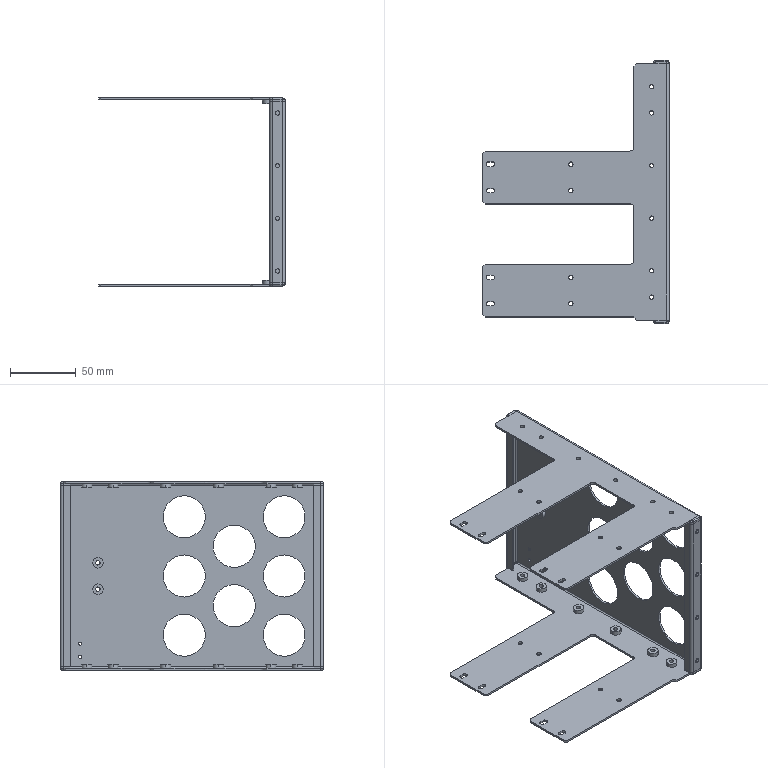Part | SolidWorks | features ICE 6, HoleWzd 5, SMWeldBead 4, EdgeFlange 2, Chamfer 1, Fillet 1, FlatPattern 1, MirrorPattern 1, SMBaseFlange 1, SheetMetal 1 | 1 solid | 433 faces | box 142 x 200 x 143 mm | volume 82962 mm3 | plane 167 | cylinder 158 | spline 104 | torus 4 | commonest cylinder face diameters 3.5 x40 3.3 x36 8 x28 32 x16 2 x12 1 x6